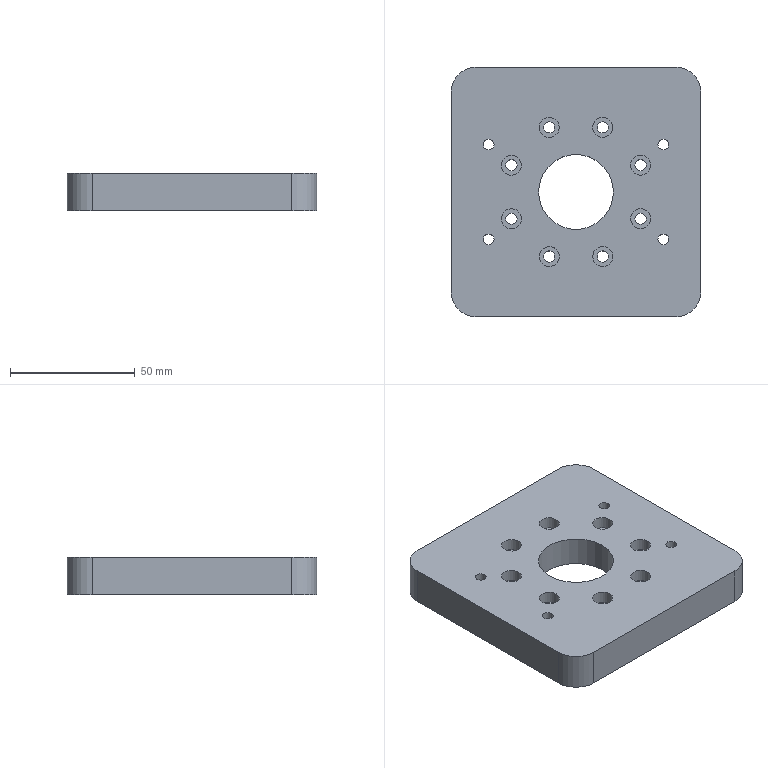Part | NX | 1 solid | 41 faces | box 100 x 100 x 15 mm | volume 127371 mm3 | cylinder 26 | plane 15 | commonest cylinder face diameters 4.5 x8 8 x8 4.3 x4 20 x4 30 x1 62.1 x1
STEP:
#1=CARTESIAN_POINT('',(-23.619,-10.715,-12.));
#2=VERTEX_POINT('',#1);
#3=CARTESIAN_POINT('',(-25.869,-10.715,-12.));
#4=DIRECTION('',(0.,0.,1.));
#5=DIRECTION('',(1.,0.,0.));
#6=AXIS2_PLACEMENT_3D('',#3,#4,#5);
#7=CIRCLE('',#6,2.25);
#8=EDGE_CURVE('',#2,#2,#7,.F.);
#9=ORIENTED_EDGE('',*,*,#8,.T.);
#10=EDGE_LOOP('',(#9));
#11=FACE_BOUND('',#10,.T.);
#12=CARTESIAN_POINT('',(-23.619,-10.715,-5.));
#13=VERTEX_POINT('',#12);
#14=CARTESIAN_POINT('',(-25.869,-10.715,-5.));
#15=DIRECTION('',(0.,0.,1.));
#16=DIRECTION('',(1.,0.,0.));
#17=AXIS2_PLACEMENT_3D('',#14,#15,#16);
#18=CIRCLE('',#17,2.25);
#19=EDGE_CURVE('',#13,#13,#18,.F.);
#20=ORIENTED_EDGE('',*,*,#19,.F.);
#21=EDGE_LOOP('',(#20));
#22=FACE_BOUND('',#21,.T.);
#23=CARTESIAN_POINT('',(-25.869,-10.715,-15.));
#24=DIRECTION('',(0.,0.,1.));
#25=DIRECTION('',(1.,0.,0.));
#26=AXIS2_PLACEMENT_3D('',#23,#24,#25);
#27=CYLINDRICAL_SURFACE('',#26,2.25);
#28=ADVANCED_FACE('',(#11,#22),#27,.F.);
#29=CARTESIAN_POINT('',(-23.619,10.715,-12.));
#30=VERTEX_POINT('',#29);
#31=CARTESIAN_POINT('',(-25.869,10.715,-12.));
#32=DIRECTION('',(0.,0.,1.));
#33=DIRECTION('',(1.,0.,0.));
#34=AXIS2_PLACEMENT_3D('',#31,#32,#33);
#35=CIRCLE('',#34,2.25);
#36=EDGE_CURVE('',#30,#30,#35,.F.);
#37=ORIENTED_EDGE('',*,*,#36,.T.);
#38=EDGE_LOOP('',(#37));
#39=FACE_BOUND('',#38,.T.);
#40=CARTESIAN_POINT('',(-23.619,10.715,-5.));
#41=VERTEX_POINT('',#40);
#42=CARTESIAN_POINT('',(-25.869,10.715,-5.));
#43=DIRECTION('',(0.,0.,1.));
#44=DIRECTION('',(1.,0.,0.));
#45=AXIS2_PLACEMENT_3D('',#42,#43,#44);
#46=CIRCLE('',#45,2.25);
#47=EDGE_CURVE('',#41,#41,#46,.F.);
#48=ORIENTED_EDGE('',*,*,#47,.F.);
#49=EDGE_LOOP('',(#48));
#50=FACE_BOUND('',#49,.T.);
#51=CARTESIAN_POINT('',(-25.869,10.715,-15.));
#52=DIRECTION('',(0.,0.,1.));
#53=DIRECTION('',(1.,0.,0.));
#54=AXIS2_PLACEMENT_3D('',#51,#52,#53);
#55=CYLINDRICAL_SURFACE('',#54,2.25);
#56=ADVANCED_FACE('',(#39,#50),#55,.F.);
#57=CARTESIAN_POINT('',(-8.465,-25.869,-12.));
#58=VERTEX_POINT('',#57);
#59=CARTESIAN_POINT('',(-10.715,-25.869,-12.));
#60=DIRECTION('',(0.,0.,1.));
#61=DIRECTION('',(1.,0.,0.));
#62=AXIS2_PLACEMENT_3D('',#59,#60,#61);
#63=CIRCLE('',#62,2.25);
#64=EDGE_CURVE('',#58,#58,#63,.F.);
#65=ORIENTED_EDGE('',*,*,#64,.T.);
#66=EDGE_LOOP('',(#65));
#67=FACE_BOUND('',#66,.T.);
#68=CARTESIAN_POINT('',(-8.465,-25.869,-5.));
#69=VERTEX_POINT('',#68);
#70=CARTESIAN_POINT('',(-10.715,-25.869,-5.));
#71=DIRECTION('',(0.,0.,1.));
#72=DIRECTION('',(1.,0.,0.));
#73=AXIS2_PLACEMENT_3D('',#70,#71,#72);
#74=CIRCLE('',#73,2.25);
#75=EDGE_CURVE('',#69,#69,#74,.F.);
#76=ORIENTED_EDGE('',*,*,#75,.F.);
#77=EDGE_LOOP('',(#76));
#78=FACE_BOUND('',#77,.T.);
#79=CARTESIAN_POINT('',(-10.715,-25.869,-15.));
#80=DIRECTION('',(0.,0.,1.));
#81=DIRECTION('',(1.,0.,0.));
#82=AXIS2_PLACEMENT_3D('',#79,#80,#81);
#83=CYLINDRICAL_SURFACE('',#82,2.25);
#84=ADVANCED_FACE('',(#67,#78),#83,.F.);
#85=CARTESIAN_POINT('',(-8.465,25.869,-12.));
#86=VERTEX_POINT('',#85);
#87=CARTESIAN_POINT('',(-10.715,25.869,-12.));
#88=DIRECTION('',(0.,0.,1.));
#89=DIRECTION('',(1.,0.,0.));
#90=AXIS2_PLACEMENT_3D('',#87,#88,#89);
#91=CIRCLE('',#90,2.25);
#92=EDGE_CURVE('',#86,#86,#91,.F.);
#93=ORIENTED_EDGE('',*,*,#92,.T.);
#94=EDGE_LOOP('',(#93));
#95=FACE_BOUND('',#94,.T.);
#96=CARTESIAN_POINT('',(-8.465,25.869,-5.));
#97=VERTEX_POINT('',#96);
#98=CARTESIAN_POINT('',(-10.715,25.869,-5.));
#99=DIRECTION('',(0.,0.,1.));
#100=DIRECTION('',(1.,0.,0.));
#101=AXIS2_PLACEMENT_3D('',#98,#99,#100);
#102=CIRCLE('',#101,2.25);
#103=EDGE_CURVE('',#97,#97,#102,.F.);
#104=ORIENTED_EDGE('',*,*,#103,.F.);
#105=EDGE_LOOP('',(#104));
#106=FACE_BOUND('',#105,.T.);
#107=CARTESIAN_POINT('',(-10.715,25.869,-15.));
#108=DIRECTION('',(0.,0.,1.));
#109=DIRECTION('',(1.,0.,0.));
#110=AXIS2_PLACEMENT_3D('',#107,#108,#109);
#111=CYLINDRICAL_SURFACE('',#110,2.25);
#112=ADVANCED_FACE('',(#95,#106),#111,.F.);
#113=CARTESIAN_POINT('',(12.965,-25.869,-12.));
#114=VERTEX_POINT('',#113);
#115=CARTESIAN_POINT('',(10.715,-25.869,-12.));
#116=DIRECTION('',(0.,0.,1.));
#117=DIRECTION('',(1.,0.,0.));
#118=AXIS2_PLACEMENT_3D('',#115,#116,#117);
#119=CIRCLE('',#118,2.25);
#120=EDGE_CURVE('',#114,#114,#119,.F.);
#121=ORIENTED_EDGE('',*,*,#120,.T.);
#122=EDGE_LOOP('',(#121));
#123=FACE_BOUND('',#122,.T.);
#124=CARTESIAN_POINT('',(12.965,-25.869,-5.));
#125=VERTEX_POINT('',#124);
#126=CARTESIAN_POINT('',(10.715,-25.869,-5.));
#127=DIRECTION('',(0.,0.,1.));
#128=DIRECTION('',(1.,0.,0.));
#129=AXIS2_PLACEMENT_3D('',#126,#127,#128);
#130=CIRCLE('',#129,2.25);
#131=EDGE_CURVE('',#125,#125,#130,.F.);
#132=ORIENTED_EDGE('',*,*,#131,.F.);
#133=EDGE_LOOP('',(#132));
#134=FACE_BOUND('',#133,.T.);
#135=CARTESIAN_POINT('',(10.715,-25.869,-15.));
#136=DIRECTION('',(0.,0.,1.));
#137=DIRECTION('',(1.,0.,0.));
#138=AXIS2_PLACEMENT_3D('',#135,#136,#137);
#139=CYLINDRICAL_SURFACE('',#138,2.25);
#140=ADVANCED_FACE('',(#123,#134),#139,.F.);
#141=CARTESIAN_POINT('',(12.965,25.869,-12.));
#142=VERTEX_POINT('',#141);
#143=CARTESIAN_POINT('',(10.715,25.869,-12.));
#144=DIRECTION('',(0.,0.,1.));
#145=DIRECTION('',(1.,0.,0.));
#146=AXIS2_PLACEMENT_3D('',#143,#144,#145);
#147=CIRCLE('',#146,2.25);
#148=EDGE_CURVE('',#142,#142,#147,.F.);
#149=ORIENTED_EDGE('',*,*,#148,.T.);
#150=EDGE_LOOP('',(#149));
#151=FACE_BOUND('',#150,.T.);
#152=CARTESIAN_POINT('',(12.965,25.869,-5.));
#153=VERTEX_POINT('',#152);
#154=CARTESIAN_POINT('',(10.715,25.869,-5.));
#155=DIRECTION('',(0.,0.,1.));
#156=DIRECTION('',(1.,0.,0.));
#157=AXIS2_PLACEMENT_3D('',#154,#155,#156);
#158=CIRCLE('',#157,2.25);
#159=EDGE_CURVE('',#153,#153,#158,.F.);
#160=ORIENTED_EDGE('',*,*,#159,.F.);
#161=EDGE_LOOP('',(#160));
#162=FACE_BOUND('',#161,.T.);
#163=CARTESIAN_POINT('',(10.715,25.869,-15.));
#164=DIRECTION('',(0.,0.,1.));
#165=DIRECTION('',(1.,0.,0.));
#166=AXIS2_PLACEMENT_3D('',#163,#164,#165);
#167=CYLINDRICAL_SURFACE('',#166,2.25);
#168=ADVANCED_FACE('',(#151,#162),#167,.F.);
#169=CARTESIAN_POINT('',(28.119,-10.715,-12.));
#170=VERTEX_POINT('',#169);
#171=CARTESIAN_POINT('',(25.869,-10.715,-12.));
#172=DIRECTION('',(0.,0.,1.));
#173=DIRECTION('',(1.,0.,0.));
#174=AXIS2_PLACEMENT_3D('',#171,#172,#173);
#175=CIRCLE('',#174,2.25);
#176=EDGE_CURVE('',#170,#170,#175,.F.);
#177=ORIENTED_EDGE('',*,*,#176,.T.);
#178=EDGE_LOOP('',(#177));
#179=FACE_BOUND('',#178,.T.);
#180=CARTESIAN_POINT('',(28.119,-10.715,-5.));
#181=VERTEX_POINT('',#180);
#182=CARTESIAN_POINT('',(25.869,-10.715,-5.));
#183=DIRECTION('',(0.,0.,1.));
#184=DIRECTION('',(1.,0.,0.));
#185=AXIS2_PLACEMENT_3D('',#182,#183,#184);
#186=CIRCLE('',#185,2.25);
#187=EDGE_CURVE('',#181,#181,#186,.F.);
#188=ORIENTED_EDGE('',*,*,#187,.F.);
#189=EDGE_LOOP('',(#188));
#190=FACE_BOUND('',#189,.T.);
#191=CARTESIAN_POINT('',(25.869,-10.715,-15.));
#192=DIRECTION('',(0.,0.,1.));
#193=DIRECTION('',(1.,0.,0.));
#194=AXIS2_PLACEMENT_3D('',#191,#192,#193);
#195=CYLINDRICAL_SURFACE('',#194,2.25);
#196=ADVANCED_FACE('',(#179,#190),#195,.F.);
#197=CARTESIAN_POINT('',(28.119,10.715,-12.));
#198=VERTEX_POINT('',#197);
#199=CARTESIAN_POINT('',(25.869,10.715,-12.));
#200=DIRECTION('',(0.,0.,1.));
#201=DIRECTION('',(1.,0.,0.));
#202=AXIS2_PLACEMENT_3D('',#199,#200,#201);
#203=CIRCLE('',#202,2.25);
#204=EDGE_CURVE('',#198,#198,#203,.F.);
#205=ORIENTED_EDGE('',*,*,#204,.T.);
#206=EDGE_LOOP('',(#205));
#207=FACE_BOUND('',#206,.T.);
#208=CARTESIAN_POINT('',(28.119,10.715,-5.));
#209=VERTEX_POINT('',#208);
#210=CARTESIAN_POINT('',(25.869,10.715,-5.));
#211=DIRECTION('',(0.,0.,1.));
#212=DIRECTION('',(1.,0.,0.));
#213=AXIS2_PLACEMENT_3D('',#210,#211,#212);
#214=CIRCLE('',#213,2.25);
#215=EDGE_CURVE('',#209,#209,#214,.F.);
#216=ORIENTED_EDGE('',*,*,#215,.F.);
#217=EDGE_LOOP('',(#216));
#218=FACE_BOUND('',#217,.T.);
#219=CARTESIAN_POINT('',(25.869,10.715,-15.));
#220=DIRECTION('',(0.,0.,1.));
#221=DIRECTION('',(1.,0.,0.));
#222=AXIS2_PLACEMENT_3D('',#219,#220,#221);
#223=CYLINDRICAL_SURFACE('',#222,2.25);
#224=ADVANCED_FACE('',(#207,#218),#223,.F.);
#225=CARTESIAN_POINT('',(-50.,-40.,0.));
#226=VERTEX_POINT('',#225);
#227=CARTESIAN_POINT('',(-50.,40.,0.));
#228=VERTEX_POINT('',#227);
#229=CARTESIAN_POINT('',(-50.,-50.,0.));
#230=DIRECTION('',(0.,1.,0.));
#231=VECTOR('',#230,1000.);
#232=LINE('',#229,#231);
#233=EDGE_CURVE('',#226,#228,#232,.T.);
#234=ORIENTED_EDGE('',*,*,#233,.T.);
#235=CARTESIAN_POINT('',(-50.,40.,-15.));
#236=VERTEX_POINT('',#235);
#237=CARTESIAN_POINT('',(-50.,40.,-15.));
#238=DIRECTION('',(0.,0.,1.));
#239=VECTOR('',#238,1000.);
#240=LINE('',#237,#239);
#241=EDGE_CURVE('',#228,#236,#240,.F.);
#242=ORIENTED_EDGE('',*,*,#241,.T.);
#243=CARTESIAN_POINT('',(-50.,-40.,-15.));
#244=VERTEX_POINT('',#243);
#245=CARTESIAN_POINT('',(-50.,-50.,-15.));
#246=DIRECTION('',(0.,1.,0.));
#247=VECTOR('',#246,1000.);
#248=LINE('',#245,#247);
#249=EDGE_CURVE('',#244,#236,#248,.T.);
#250=ORIENTED_EDGE('',*,*,#249,.F.);
#251=CARTESIAN_POINT('',(-50.,-40.,-15.));
#252=DIRECTION('',(0.,0.,1.));
#253=VECTOR('',#252,1000.);
#254=LINE('',#251,#253);
#255=EDGE_CURVE('',#244,#226,#254,.T.);
#256=ORIENTED_EDGE('',*,*,#255,.T.);
#257=EDGE_LOOP('',(#234,#242,#250,#256));
#258=FACE_BOUND('',#257,.T.);
#259=CARTESIAN_POINT('',(-50.,-50.,-15.));
#260=DIRECTION('',(1.,0.,0.));
#261=DIRECTION('',(0.,0.,-1.));
#262=AXIS2_PLACEMENT_3D('',#259,#260,#261);
#263=PLANE('',#262);
#264=ADVANCED_FACE('',(#258),#263,.F.);
#265=CARTESIAN_POINT('',(-40.,50.,-15.));
#266=VERTEX_POINT('',#265);
#267=CARTESIAN_POINT('',(40.,50.,-15.));
#268=VERTEX_POINT('',#267);
#269=CARTESIAN_POINT('',(-50.,50.,-15.));
#270=DIRECTION('',(1.,0.,0.));
#271=VECTOR('',#270,1000.);
#272=LINE('',#269,#271);
#273=EDGE_CURVE('',#266,#268,#272,.T.);
#274=ORIENTED_EDGE('',*,*,#273,.F.);
#275=CARTESIAN_POINT('',(-40.,50.,0.));
#276=VERTEX_POINT('',#275);
#277=CARTESIAN_POINT('',(-40.,50.,-15.));
#278=DIRECTION('',(0.,0.,1.));
#279=VECTOR('',#278,1000.);
#280=LINE('',#277,#279);
#281=EDGE_CURVE('',#266,#276,#280,.T.);
#282=ORIENTED_EDGE('',*,*,#281,.T.);
#283=CARTESIAN_POINT('',(40.,50.,0.));
#284=VERTEX_POINT('',#283);
#285=CARTESIAN_POINT('',(-50.,50.,0.));
#286=DIRECTION('',(1.,0.,0.));
#287=VECTOR('',#286,1000.);
#288=LINE('',#285,#287);
#289=EDGE_CURVE('',#276,#284,#288,.T.);
#290=ORIENTED_EDGE('',*,*,#289,.T.);
#291=CARTESIAN_POINT('',(40.,50.,-15.));
#292=DIRECTION('',(0.,0.,1.));
#293=VECTOR('',#292,1000.);
#294=LINE('',#291,#293);
#295=EDGE_CURVE('',#284,#268,#294,.F.);
#296=ORIENTED_EDGE('',*,*,#295,.T.);
#297=EDGE_LOOP('',(#274,#282,#290,#296));
#298=FACE_BOUND('',#297,.T.);
#299=CARTESIAN_POINT('',(-50.,50.,-15.));
#300=DIRECTION('',(0.,-1.,0.));
#301=DIRECTION('',(1.,0.,0.));
#302=AXIS2_PLACEMENT_3D('',#299,#300,#301);
#303=PLANE('',#302);
#304=ADVANCED_FACE('',(#298),#303,.F.);
#305=CARTESIAN_POINT('',(50.,40.,-15.));
#306=VERTEX_POINT('',#305);
#307=CARTESIAN_POINT('',(50.,-40.,-15.));
#308=VERTEX_POINT('',#307);
#309=CARTESIAN_POINT('',(50.,50.,-15.));
#310=DIRECTION('',(0.,-1.,0.));
#311=VECTOR('',#310,1000.);
#312=LINE('',#309,#311);
#313=EDGE_CURVE('',#306,#308,#312,.T.);
#314=ORIENTED_EDGE('',*,*,#313,.F.);
#315=CARTESIAN_POINT('',(50.,40.,0.));
#316=VERTEX_POINT('',#315);
#317=CARTESIAN_POINT('',(50.,40.,-15.));
#318=DIRECTION('',(0.,0.,1.));
#319=VECTOR('',#318,1000.);
#320=LINE('',#317,#319);
#321=EDGE_CURVE('',#306,#316,#320,.T.);
#322=ORIENTED_EDGE('',*,*,#321,.T.);
#323=CARTESIAN_POINT('',(50.,-40.,0.));
#324=VERTEX_POINT('',#323);
#325=CARTESIAN_POINT('',(50.,50.,0.));
#326=DIRECTION('',(0.,-1.,0.));
#327=VECTOR('',#326,1000.);
#328=LINE('',#325,#327);
#329=EDGE_CURVE('',#316,#324,#328,.T.);
#330=ORIENTED_EDGE('',*,*,#329,.T.);
#331=CARTESIAN_POINT('',(50.,-40.,-15.));
#332=DIRECTION('',(0.,0.,1.));
#333=VECTOR('',#332,1000.);
#334=LINE('',#331,#333);
#335=EDGE_CURVE('',#324,#308,#334,.F.);
#336=ORIENTED_EDGE('',*,*,#335,.T.);
#337=EDGE_LOOP('',(#314,#322,#330,#336));
#338=FACE_BOUND('',#337,.T.);
#339=CARTESIAN_POINT('',(50.,50.,-15.));
#340=DIRECTION('',(-1.,0.,0.));
#341=DIRECTION('',(0.,0.,1.));
#342=AXIS2_PLACEMENT_3D('',#339,#340,#341);
#343=PLANE('',#342);
#344=ADVANCED_FACE('',(#338),#343,.F.);
#345=CARTESIAN_POINT('',(-32.85,19.,-15.));
#346=VERTEX_POINT('',#345);
#347=CARTESIAN_POINT('',(-35.,19.,-15.));
#348=DIRECTION('',(0.,0.,1.));
#349=DIRECTION('',(1.,0.,0.));
#350=AXIS2_PLACEMENT_3D('',#347,#348,#349);
#351=CIRCLE('',#350,2.15);
#352=EDGE_CURVE('',#346,#346,#351,.T.);
#353=ORIENTED_EDGE('',*,*,#352,.F.);
#354=EDGE_LOOP('',(#353));
#355=FACE_BOUND('',#354,.T.);
#356=CARTESIAN_POINT('',(-32.85,19.,0.));
#357=VERTEX_POINT('',#356);
#358=CARTESIAN_POINT('',(-35.,19.,0.));
#359=DIRECTION('',(0.,0.,1.));
#360=DIRECTION('',(1.,0.,0.));
#361=AXIS2_PLACEMENT_3D('',#358,#359,#360);
#362=CIRCLE('',#361,2.15);
#363=EDGE_CURVE('',#357,#357,#362,.T.);
#364=ORIENTED_EDGE('',*,*,#363,.T.);
#365=EDGE_LOOP('',(#364));
#366=FACE_BOUND('',#365,.T.);
#367=CARTESIAN_POINT('',(-35.,19.,-15.));
#368=DIRECTION('',(0.,0.,1.));
#369=DIRECTION('',(1.,0.,0.));
#370=AXIS2_PLACEMENT_3D('',#367,#368,#369);
#371=CYLINDRICAL_SURFACE('',#370,2.15);
#372=ADVANCED_FACE('',(#355,#366),#371,.F.);
#373=CARTESIAN_POINT('',(15.,0.,-12.));
#374=VERTEX_POINT('',#373);
#375=CARTESIAN_POINT('',(0.,0.,-12.));
#376=DIRECTION('',(0.,0.,1.));
#377=DIRECTION('',(1.,0.,0.));
#378=AXIS2_PLACEMENT_3D('',#375,#376,#377);
#379=CIRCLE('',#378,15.);
#380=EDGE_CURVE('',#374,#374,#379,.F.);
#381=ORIENTED_EDGE('',*,*,#380,.T.);
#382=EDGE_LOOP('',(#381));
#383=FACE_BOUND('',#382,.T.);
#384=CARTESIAN_POINT('',(15.,0.,0.));
#385=VERTEX_POINT('',#384);
#386=CARTESIAN_POINT('',(0.,0.,0.));
#387=DIRECTION('',(0.,0.,1.));
#388=DIRECTION('',(1.,0.,0.));
#389=AXIS2_PLACEMENT_3D('',#386,#387,#388);
#390=CIRCLE('',#389,15.);
#391=EDGE_CURVE('',#385,#385,#390,.T.);
#392=ORIENTED_EDGE('',*,*,#391,.T.);
#393=EDGE_LOOP('',(#392));
#394=FACE_BOUND('',#393,.T.);
#395=CARTESIAN_POINT('',(0.,0.,-15.));
#396=DIRECTION('',(0.,0.,1.));
#397=DIRECTION('',(1.,0.,0.));
#398=AXIS2_PLACEMENT_3D('',#395,#396,#397);
#399=CYLINDRICAL_SURFACE('',#398,15.);
#400=ADVANCED_FACE('',(#383,#394),#399,.F.);
#401=CARTESIAN_POINT('',(37.15,-19.,-15.));
#402=VERTEX_POINT('',#401);
#403=CARTESIAN_POINT('',(35.,-19.,-15.));
#404=DIRECTION('',(0.,0.,1.));
#405=DIRECTION('',(1.,0.,0.));
#406=AXIS2_PLACEMENT_3D('',#403,#404,#405);
#407=CIRCLE('',#406,2.15);
#408=EDGE_CURVE('',#402,#402,#407,.T.);
#409=ORIENTED_EDGE('',*,*,#408,.F.);
#410=EDGE_LOOP('',(#409));
#411=FACE_BOUND('',#410,.T.);
#412=CARTESIAN_POINT('',(37.15,-19.,0.));
#413=VERTEX_POINT('',#412);
#414=CARTESIAN_POINT('',(35.,-19.,0.));
#415=DIRECTION('',(0.,0.,1.));
#416=DIRECTION('',(1.,0.,0.));
#417=AXIS2_PLACEMENT_3D('',#414,#415,#416);
#418=CIRCLE('',#417,2.15);
#419=EDGE_CURVE('',#413,#413,#418,.T.);
#420=ORIENTED_EDGE('',*,*,#419,.T.);
#421=EDGE_LOOP('',(#420));
#422=FACE_BOUND('',#421,.T.);
#423=CARTESIAN_POINT('',(35.,-19.,-15.));
#424=DIRECTION('',(0.,0.,1.));
#425=DIRECTION('',(1.,0.,0.));
#426=AXIS2_PLACEMENT_3D('',#423,#424,#425);
#427=CYLINDRICAL_SURFACE('',#426,2.15);
#428=ADVANCED_FACE('',(#411,#422),#427,.F.);
#429=CARTESIAN_POINT('',(37.15,19.,-15.));
#430=VERTEX_POINT('',#429);
#431=CARTESIAN_POINT('',(35.,19.,-15.));
#432=DIRECTION('',(0.,0.,1.));
#433=DIRECTION('',(1.,0.,0.));
#434=AXIS2_PLACEMENT_3D('',#431,#432,#433);
#435=CIRCLE('',#434,2.15);
#436=EDGE_CURVE('',#430,#430,#435,.T.);
#437=ORIENTED_EDGE('',*,*,#436,.F.);
#438=EDGE_LOOP('',(#437));
#439=FACE_BOUND('',#438,.T.);
#440=CARTESIAN_POINT('',(37.15,19.,0.));
#441=VERTEX_POINT('',#440);
#442=CARTESIAN_POINT('',(35.,19.,0.));
#443=DIRECTION('',(0.,0.,1.));
#444=DIRECTION('',(1.,0.,0.));
#445=AXIS2_PLACEMENT_3D('',#442,#443,#444);
#446=CIRCLE('',#445,2.15);
#447=EDGE_CURVE('',#441,#441,#446,.T.);
#448=ORIENTED_EDGE('',*,*,#447,.T.);
#449=EDGE_LOOP('',(#448));
#450=FACE_BOUND('',#449,.T.);
#451=CARTESIAN_POINT('',(35.,19.,-15.));
#452=DIRECTION('',(0.,0.,1.));
#453=DIRECTION('',(1.,0.,0.));
#454=AXIS2_PLACEMENT_3D('',#451,#452,#453);
#455=CYLINDRICAL_SURFACE('',#454,2.15);
#456=ADVANCED_FACE('',(#439,#450),#455,.F.);
#457=CARTESIAN_POINT('',(40.,-50.,0.));
#458=VERTEX_POINT('',#457);
#459=CARTESIAN_POINT('',(-40.,-50.,0.));
#460=VERTEX_POINT('',#459);
#461=CARTESIAN_POINT('',(50.,-50.,0.));
#462=DIRECTION('',(-1.,0.,0.));
#463=VECTOR('',#462,1000.);
#464=LINE('',#461,#463);
#465=EDGE_CURVE('',#458,#460,#464,.T.);
#466=ORIENTED_EDGE('',*,*,#465,.T.);
#467=CARTESIAN_POINT('',(-40.,-50.,-15.));
#468=VERTEX_POINT('',#467);
#469=CARTESIAN_POINT('',(-40.,-50.,-15.));
#470=DIRECTION('',(0.,0.,1.));
#471=VECTOR('',#470,1000.);
#472=LINE('',#469,#471);
#473=EDGE_CURVE('',#460,#468,#472,.F.);
#474=ORIENTED_EDGE('',*,*,#473,.T.);
#475=CARTESIAN_POINT('',(40.,-50.,-15.));
#476=VERTEX_POINT('',#475);
#477=CARTESIAN_POINT('',(50.,-50.,-15.));
#478=DIRECTION('',(-1.,0.,0.));
#479=VECTOR('',#478,1000.);
#480=LINE('',#477,#479);
#481=EDGE_CURVE('',#476,#468,#480,.T.);
#482=ORIENTED_EDGE('',*,*,#481,.F.);
#483=CARTESIAN_POINT('',(40.,-50.,-15.));
#484=DIRECTION('',(0.,0.,1.));
#485=VECTOR('',#484,1000.);
#486=LINE('',#483,#485);
#487=EDGE_CURVE('',#476,#458,#486,.T.);
#488=ORIENTED_EDGE('',*,*,#487,.T.);
#489=EDGE_LOOP('',(#466,#474,#482,#488));
#490=FACE_BOUND('',#489,.T.);
#491=CARTESIAN_POINT('',(50.,-50.,-15.));
#492=DIRECTION('',(0.,1.,0.));
#493=DIRECTION('',(-1.,0.,0.));
#494=AXIS2_PLACEMENT_3D('',#491,#492,#493);
#495=PLANE('',#494);
#496=ADVANCED_FACE('',(#490),#495,.F.);
#497=CARTESIAN_POINT('',(-32.85,-19.,-15.));
#498=VERTEX_POINT('',#497);
#499=CARTESIAN_POINT('',(-35.,-19.,-15.));
#500=DIRECTION('',(0.,0.,1.));
#501=DIRECTION('',(1.,0.,0.));
#502=AXIS2_PLACEMENT_3D('',#499,#500,#501);
#503=CIRCLE('',#502,2.15);
#504=EDGE_CURVE('',#498,#498,#503,.T.);
#505=ORIENTED_EDGE('',*,*,#504,.F.);
#506=EDGE_LOOP('',(#505));
#507=FACE_BOUND('',#506,.T.);
#508=CARTESIAN_POINT('',(-32.85,-19.,0.));
#509=VERTEX_POINT('',#508);
#510=CARTESIAN_POINT('',(-35.,-19.,0.));
#511=DIRECTION('',(0.,0.,1.));
#512=DIRECTION('',(1.,0.,0.));
#513=AXIS2_PLACEMENT_3D('',#510,#511,#512);
#514=CIRCLE('',#513,2.15);
#515=EDGE_CURVE('',#509,#509,#514,.T.);
#516=ORIENTED_EDGE('',*,*,#515,.T.);
#517=EDGE_LOOP('',(#516));
#518=FACE_BOUND('',#517,.T.);
#519=CARTESIAN_POINT('',(-35.,-19.,-15.));
#520=DIRECTION('',(0.,0.,1.));
#521=DIRECTION('',(1.,0.,0.));
#522=AXIS2_PLACEMENT_3D('',#519,#520,#521);
#523=CYLINDRICAL_SURFACE('',#522,2.15);
#524=ADVANCED_FACE('',(#507,#518),#523,.F.);
#525=CARTESIAN_POINT('',(31.05,0.,-15.));
#526=VERTEX_POINT('',#525);
#527=CARTESIAN_POINT('',(0.,0.,-15.));
#528=DIRECTION('',(0.,0.,1.));
#529=DIRECTION('',(1.,0.,0.));
#530=AXIS2_PLACEMENT_3D('',#527,#528,#529);
#531=CIRCLE('',#530,31.05);
#532=EDGE_CURVE('',#526,#526,#531,.T.);
#533=ORIENTED_EDGE('',*,*,#532,.T.);
#534=EDGE_LOOP('',(#533));
#535=FACE_BOUND('',#534,.T.);
#536=ORIENTED_EDGE('',*,*,#249,.T.);
#537=CARTESIAN_POINT('',(-40.,40.,-15.));
#538=DIRECTION('',(0.,0.,1.));
#539=DIRECTION('',(1.,0.,0.));
#540=AXIS2_PLACEMENT_3D('',#537,#538,#539);
#541=CIRCLE('',#540,10.);
#542=EDGE_CURVE('',#236,#266,#541,.F.);
#543=ORIENTED_EDGE('',*,*,#542,.T.);
#544=ORIENTED_EDGE('',*,*,#273,.T.);
#545=CARTESIAN_POINT('',(40.,40.,-15.));
#546=DIRECTION('',(0.,0.,1.));
#547=DIRECTION('',(1.,0.,0.));
#548=AXIS2_PLACEMENT_3D('',#545,#546,#547);
#549=CIRCLE('',#548,10.);
#550=EDGE_CURVE('',#268,#306,#549,.F.);
#551=ORIENTED_EDGE('',*,*,#550,.T.);
#552=ORIENTED_EDGE('',*,*,#313,.T.);
#553=CARTESIAN_POINT('',(40.,-40.,-15.));
#554=DIRECTION('',(0.,0.,1.));
#555=DIRECTION('',(1.,0.,0.));
#556=AXIS2_PLACEMENT_3D('',#553,#554,#555);
#557=CIRCLE('',#556,10.);
#558=EDGE_CURVE('',#308,#476,#557,.F.);
#559=ORIENTED_EDGE('',*,*,#558,.T.);
#560=ORIENTED_EDGE('',*,*,#481,.T.);
#561=CARTESIAN_POINT('',(-40.,-40.,-15.));
#562=DIRECTION('',(0.,0.,1.));
#563=DIRECTION('',(1.,0.,0.));
#564=AXIS2_PLACEMENT_3D('',#561,#562,#563);
#565=CIRCLE('',#564,10.);
#566=EDGE_CURVE('',#468,#244,#565,.F.);
#567=ORIENTED_EDGE('',*,*,#566,.T.);
#568=EDGE_LOOP('',(#536,#543,#544,#551,#552,#559,#560,#567));
#569=FACE_BOUND('',#568,.T.);
#570=ORIENTED_EDGE('',*,*,#436,.T.);
#571=EDGE_LOOP('',(#570));
#572=FACE_BOUND('',#571,.T.);
#573=ORIENTED_EDGE('',*,*,#408,.T.);
#574=EDGE_LOOP('',(#573));
#575=FACE_BOUND('',#574,.T.);
#576=ORIENTED_EDGE('',*,*,#352,.T.);
#577=EDGE_LOOP('',(#576));
#578=FACE_BOUND('',#577,.T.);
#579=ORIENTED_EDGE('',*,*,#504,.T.);
#580=EDGE_LOOP('',(#579));
#581=FACE_BOUND('',#580,.T.);
#582=CARTESIAN_POINT('',(35.,19.,-15.));
#583=DIRECTION('',(0.,0.,1.));
#584=DIRECTION('',(1.,0.,0.));
#585=AXIS2_PLACEMENT_3D('',#582,#583,#584);
#586=PLANE('',#585);
#587=ADVANCED_FACE('',(#535,#569,#572,#575,#578,#581),#586,.F.);
#588=CARTESIAN_POINT('',(-10.715,21.869,0.));
#589=VERTEX_POINT('',#588);
#590=CARTESIAN_POINT('',(-10.715,25.869,0.));
#591=DIRECTION('',(0.,0.,1.));
#592=DIRECTION('',(0.,-1.,0.));
#593=AXIS2_PLACEMENT_3D('',#590,#591,#592);
#594=CIRCLE('',#593,4.);
#595=EDGE_CURVE('',#589,#589,#594,.T.);
#596=ORIENTED_EDGE('',*,*,#595,.F.);
#597=EDGE_LOOP('',(#596));
#598=FACE_BOUND('',#597,.T.);
#599=CARTESIAN_POINT('',(10.715,-21.869,0.));
#600=VERTEX_POINT('',#599);
#601=CARTESIAN_POINT('',(10.715,-25.869,0.));
#602=DIRECTION('',(0.,0.,1.));
#603=DIRECTION('',(0.,1.,0.));
#604=AXIS2_PLACEMENT_3D('',#601,#602,#603);
#605=CIRCLE('',#604,4.);
#606=EDGE_CURVE('',#600,#600,#605,.T.);
#607=ORIENTED_EDGE('',*,*,#606,.F.);
#608=EDGE_LOOP('',(#607));
#609=FACE_BOUND('',#608,.T.);
#610=CARTESIAN_POINT('',(7.887,23.04,0.));
#611=VERTEX_POINT('',#610);
#612=CARTESIAN_POINT('',(10.715,25.869,0.));
#613=DIRECTION('',(0.,0.,1.));
#614=DIRECTION('',(-0.7071,-0.7071,0.));
#615=AXIS2_PLACEMENT_3D('',#612,#613,#614);
#616=CIRCLE('',#615,4.);
#617=EDGE_CURVE('',#611,#611,#616,.T.);
#618=ORIENTED_EDGE('',*,*,#617,.F.);
#619=EDGE_LOOP('',(#618));
#620=FACE_BOUND('',#619,.T.);
#621=CARTESIAN_POINT('',(23.04,-7.887,0.));
#622=VERTEX_POINT('',#621);
#623=CARTESIAN_POINT('',(25.869,-10.715,0.));
#624=DIRECTION('',(0.,0.,1.));
#625=DIRECTION('',(-0.7071,0.7071,0.));
#626=AXIS2_PLACEMENT_3D('',#623,#624,#625);
#627=CIRCLE('',#626,4.);
#628=EDGE_CURVE('',#622,#622,#627,.T.);
#629=ORIENTED_EDGE('',*,*,#628,.F.);
#630=EDGE_LOOP('',(#629));
#631=FACE_BOUND('',#630,.T.);
#632=CARTESIAN_POINT('',(-21.869,-10.715,0.));
#633=VERTEX_POINT('',#632);
#634=CARTESIAN_POINT('',(-25.869,-10.715,0.));
#635=DIRECTION('',(0.,0.,1.));
#636=DIRECTION('',(1.,0.,0.));
#637=AXIS2_PLACEMENT_3D('',#634,#635,#636);
#638=CIRCLE('',#637,4.);
#639=EDGE_CURVE('',#633,#633,#638,.T.);
#640=ORIENTED_EDGE('',*,*,#639,.F.);
#641=EDGE_LOOP('',(#640));
#642=FACE_BOUND('',#641,.T.);
#643=CARTESIAN_POINT('',(-23.04,7.887,0.));
#644=VERTEX_POINT('',#643);
#645=CARTESIAN_POINT('',(-25.869,10.715,0.));
#646=DIRECTION('',(0.,0.,1.));
#647=DIRECTION('',(0.7071,-0.7071,0.));
#648=AXIS2_PLACEMENT_3D('',#645,#646,#647);
#649=CIRCLE('',#648,4.);
#650=EDGE_CURVE('',#644,#644,#649,.T.);
#651=ORIENTED_EDGE('',*,*,#650,.F.);
#652=EDGE_LOOP('',(#651));
#653=FACE_BOUND('',#652,.T.);
#654=CARTESIAN_POINT('',(-7.887,-23.04,0.));
#655=VERTEX_POINT('',#654);
#656=CARTESIAN_POINT('',(-10.715,-25.869,0.));
#657=DIRECTION('',(0.,0.,1.));
#658=DIRECTION('',(0.7071,0.7071,0.));
#659=AXIS2_PLACEMENT_3D('',#656,#657,#658);
#660=CIRCLE('',#659,4.);
#661=EDGE_CURVE('',#655,#655,#660,.T.);
#662=ORIENTED_EDGE('',*,*,#661,.F.);
#663=EDGE_LOOP('',(#662));
#664=FACE_BOUND('',#663,.T.);
#665=CARTESIAN_POINT('',(21.869,10.715,0.));
#666=VERTEX_POINT('',#665);
#667=CARTESIAN_POINT('',(25.869,10.715,0.));
#668=DIRECTION('',(0.,0.,1.));
#669=DIRECTION('',(-1.,0.,0.));
#670=AXIS2_PLACEMENT_3D('',#667,#668,#669);
#671=CIRCLE('',#670,4.);
#672=EDGE_CURVE('',#666,#666,#671,.T.);
#673=ORIENTED_EDGE('',*,*,#672,.F.);
#674=EDGE_LOOP('',(#673));
#675=FACE_BOUND('',#674,.T.);
#676=ORIENTED_EDGE('',*,*,#289,.F.);
#677=CARTESIAN_POINT('',(-40.,40.,0.));
#678=DIRECTION('',(0.,0.,1.));
#679=DIRECTION('',(1.,0.,0.));
#680=AXIS2_PLACEMENT_3D('',#677,#678,#679);
#681=CIRCLE('',#680,10.);
#682=EDGE_CURVE('',#276,#228,#681,.T.);
#683=ORIENTED_EDGE('',*,*,#682,.T.);
#684=ORIENTED_EDGE('',*,*,#233,.F.);
#685=CARTESIAN_POINT('',(-40.,-40.,0.));
#686=DIRECTION('',(0.,0.,1.));
#687=DIRECTION('',(1.,0.,0.));
#688=AXIS2_PLACEMENT_3D('',#685,#686,#687);
#689=CIRCLE('',#688,10.);
#690=EDGE_CURVE('',#226,#460,#689,.T.);
#691=ORIENTED_EDGE('',*,*,#690,.T.);
#692=ORIENTED_EDGE('',*,*,#465,.F.);
#693=CARTESIAN_POINT('',(40.,-40.,0.));
#694=DIRECTION('',(0.,0.,1.));
#695=DIRECTION('',(1.,0.,0.));
#696=AXIS2_PLACEMENT_3D('',#693,#694,#695);
#697=CIRCLE('',#696,10.);
#698=EDGE_CURVE('',#458,#324,#697,.T.);
#699=ORIENTED_EDGE('',*,*,#698,.T.);
#700=ORIENTED_EDGE('',*,*,#329,.F.);
#701=CARTESIAN_POINT('',(40.,40.,0.));
#702=DIRECTION('',(0.,0.,1.));
#703=DIRECTION('',(1.,0.,0.));
#704=AXIS2_PLACEMENT_3D('',#701,#702,#703);
#705=CIRCLE('',#704,10.);
#706=EDGE_CURVE('',#316,#284,#705,.T.);
#707=ORIENTED_EDGE('',*,*,#706,.T.);
#708=EDGE_LOOP('',(#676,#683,#684,#691,#692,#699,#700,#707));
#709=FACE_BOUND('',#708,.T.);
#710=ORIENTED_EDGE('',*,*,#447,.F.);
#711=EDGE_LOOP('',(#710));
#712=FACE_BOUND('',#711,.T.);
#713=ORIENTED_EDGE('',*,*,#419,.F.);
#714=EDGE_LOOP('',(#713));
#715=FACE_BOUND('',#714,.T.);
#716=ORIENTED_EDGE('',*,*,#391,.F.);
#717=EDGE_LOOP('',(#716));
#718=FACE_BOUND('',#717,.T.);
#719=ORIENTED_EDGE('',*,*,#363,.F.);
#720=EDGE_LOOP('',(#719));
#721=FACE_BOUND('',#720,.T.);
#722=ORIENTED_EDGE('',*,*,#515,.F.);
#723=EDGE_LOOP('',(#722));
#724=FACE_BOUND('',#723,.T.);
#725=CARTESIAN_POINT('',(35.,19.,0.));
#726=DIRECTION('',(0.,0.,1.));
#727=DIRECTION('',(1.,0.,0.));
#728=AXIS2_PLACEMENT_3D('',#725,#726,#727);
#729=PLANE('',#728);
#730=ADVANCED_FACE('',(#598,#609,#620,#631,#642,#653,#664,#675,#709,#712,#715,#718,#721,#724),#729,.T.);
#731=CARTESIAN_POINT('',(21.869,10.715,-5.));
#732=VERTEX_POINT('',#731);
#733=CARTESIAN_POINT('',(25.869,10.715,-5.));
#734=DIRECTION('',(0.,0.,1.));
#735=DIRECTION('',(-1.,0.,0.));
#736=AXIS2_PLACEMENT_3D('',#733,#734,#735);
#737=CIRCLE('',#736,4.);
#738=EDGE_CURVE('',#732,#732,#737,.F.);
#739=ORIENTED_EDGE('',*,*,#738,.F.);
#740=EDGE_LOOP('',(#739));
#741=FACE_BOUND('',#740,.T.);
#742=ORIENTED_EDGE('',*,*,#215,.T.);
#743=EDGE_LOOP('',(#742));
#744=FACE_BOUND('',#743,.T.);
#745=CARTESIAN_POINT('',(25.869,10.715,-5.));
#746=DIRECTION('',(0.,0.,1.));
#747=DIRECTION('',(1.,0.,0.));
#748=AXIS2_PLACEMENT_3D('',#745,#746,#747);
#749=PLANE('',#748);
#750=ADVANCED_FACE('',(#741,#744),#749,.T.);
#751=ORIENTED_EDGE('',*,*,#738,.T.);
#752=EDGE_LOOP('',(#751));
#753=FACE_BOUND('',#752,.T.);
#754=ORIENTED_EDGE('',*,*,#672,.T.);
#755=EDGE_LOOP('',(#754));
#756=FACE_BOUND('',#755,.T.);
#757=CARTESIAN_POINT('',(25.869,10.715,-5.));
#758=DIRECTION('',(0.,0.,1.));
#759=DIRECTION('',(1.,0.,0.));
#760=AXIS2_PLACEMENT_3D('',#757,#758,#759);
#761=CYLINDRICAL_SURFACE('',#760,4.);
#762=ADVANCED_FACE('',(#753,#756),#761,.F.);
#763=CARTESIAN_POINT('',(-7.887,-23.04,-5.));
#764=VERTEX_POINT('',#763);
#765=CARTESIAN_POINT('',(-10.715,-25.869,-5.));
#766=DIRECTION('',(0.,0.,1.));
#767=DIRECTION('',(0.7071,0.7071,0.));
#768=AXIS2_PLACEMENT_3D('',#765,#766,#767);
#769=CIRCLE('',#768,4.);
#770=EDGE_CURVE('',#764,#764,#769,.F.);
#771=ORIENTED_EDGE('',*,*,#770,.F.);
#772=EDGE_LOOP('',(#771));
#773=FACE_BOUND('',#772,.T.);
#774=ORIENTED_EDGE('',*,*,#75,.T.);
#775=EDGE_LOOP('',(#774));
#776=FACE_BOUND('',#775,.T.);
#777=CARTESIAN_POINT('',(-10.715,-25.869,-5.));
#778=DIRECTION('',(0.,0.,1.));
#779=DIRECTION('',(1.,0.,0.));
#780=AXIS2_PLACEMENT_3D('',#777,#778,#779);
#781=PLANE('',#780);
#782=ADVANCED_FACE('',(#773,#776),#781,.T.);
#783=ORIENTED_EDGE('',*,*,#770,.T.);
#784=EDGE_LOOP('',(#783));
#785=FACE_BOUND('',#784,.T.);
#786=ORIENTED_EDGE('',*,*,#661,.T.);
#787=EDGE_LOOP('',(#786));
#788=FACE_BOUND('',#787,.T.);
#789=CARTESIAN_POINT('',(-10.715,-25.869,-5.));
#790=DIRECTION('',(0.,0.,1.));
#791=DIRECTION('',(1.,0.,0.));
#792=AXIS2_PLACEMENT_3D('',#789,#790,#791);
#793=CYLINDRICAL_SURFACE('',#792,4.);
#794=ADVANCED_FACE('',(#785,#788),#793,.F.);
#795=CARTESIAN_POINT('',(-23.04,7.887,-5.));
#796=VERTEX_POINT('',#795);
#797=CARTESIAN_POINT('',(-25.869,10.715,-5.));
#798=DIRECTION('',(0.,0.,1.));
#799=DIRECTION('',(0.7071,-0.7071,0.));
#800=AXIS2_PLACEMENT_3D('',#797,#798,#799);
#801=CIRCLE('',#800,4.);
#802=EDGE_CURVE('',#796,#796,#801,.F.);
#803=ORIENTED_EDGE('',*,*,#802,.F.);
#804=EDGE_LOOP('',(#803));
#805=FACE_BOUND('',#804,.T.);
#806=ORIENTED_EDGE('',*,*,#47,.T.);
#807=EDGE_LOOP('',(#806));
#808=FACE_BOUND('',#807,.T.);
#809=CARTESIAN_POINT('',(-25.869,10.715,-5.));
#810=DIRECTION('',(0.,0.,1.));
#811=DIRECTION('',(1.,0.,0.));
#812=AXIS2_PLACEMENT_3D('',#809,#810,#811);
#813=PLANE('',#812);
#814=ADVANCED_FACE('',(#805,#808),#813,.T.);
#815=ORIENTED_EDGE('',*,*,#802,.T.);
#816=EDGE_LOOP('',(#815));
#817=FACE_BOUND('',#816,.T.);
#818=ORIENTED_EDGE('',*,*,#650,.T.);
#819=EDGE_LOOP('',(#818));
#820=FACE_BOUND('',#819,.T.);
#821=CARTESIAN_POINT('',(-25.869,10.715,-5.));
#822=DIRECTION('',(0.,0.,1.));
#823=DIRECTION('',(1.,0.,0.));
#824=AXIS2_PLACEMENT_3D('',#821,#822,#823);
#825=CYLINDRICAL_SURFACE('',#824,4.);
#826=ADVANCED_FACE('',(#817,#820),#825,.F.);
#827=CARTESIAN_POINT('',(-21.869,-10.715,-5.));
#828=VERTEX_POINT('',#827);
#829=CARTESIAN_POINT('',(-25.869,-10.715,-5.));
#830=DIRECTION('',(0.,0.,1.));
#831=DIRECTION('',(1.,0.,0.));
#832=AXIS2_PLACEMENT_3D('',#829,#830,#831);
#833=CIRCLE('',#832,4.);
#834=EDGE_CURVE('',#828,#828,#833,.F.);
#835=ORIENTED_EDGE('',*,*,#834,.F.);
#836=EDGE_LOOP('',(#835));
#837=FACE_BOUND('',#836,.T.);
#838=ORIENTED_EDGE('',*,*,#19,.T.);
#839=EDGE_LOOP('',(#838));
#840=FACE_BOUND('',#839,.T.);
#841=CARTESIAN_POINT('',(-25.869,-10.715,-5.));
#842=DIRECTION('',(0.,0.,1.));
#843=DIRECTION('',(1.,0.,0.));
#844=AXIS2_PLACEMENT_3D('',#841,#842,#843);
#845=PLANE('',#844);
#846=ADVANCED_FACE('',(#837,#840),#845,.T.);
#847=ORIENTED_EDGE('',*,*,#834,.T.);
#848=EDGE_LOOP('',(#847));
#849=FACE_BOUND('',#848,.T.);
#850=ORIENTED_EDGE('',*,*,#639,.T.);
#851=EDGE_LOOP('',(#850));
#852=FACE_BOUND('',#851,.T.);
#853=CARTESIAN_POINT('',(-25.869,-10.715,-5.));
#854=DIRECTION('',(0.,0.,1.));
#855=DIRECTION('',(1.,0.,0.));
#856=AXIS2_PLACEMENT_3D('',#853,#854,#855);
#857=CYLINDRICAL_SURFACE('',#856,4.);
#858=ADVANCED_FACE('',(#849,#852),#857,.F.);
#859=CARTESIAN_POINT('',(23.04,-7.887,-5.));
#860=VERTEX_POINT('',#859);
#861=CARTESIAN_POINT('',(25.869,-10.715,-5.));
#862=DIRECTION('',(0.,0.,1.));
#863=DIRECTION('',(-0.7071,0.7071,0.));
#864=AXIS2_PLACEMENT_3D('',#861,#862,#863);
#865=CIRCLE('',#864,4.);
#866=EDGE_CURVE('',#860,#860,#865,.F.);
#867=ORIENTED_EDGE('',*,*,#866,.F.);
#868=EDGE_LOOP('',(#867));
#869=FACE_BOUND('',#868,.T.);
#870=ORIENTED_EDGE('',*,*,#187,.T.);
#871=EDGE_LOOP('',(#870));
#872=FACE_BOUND('',#871,.T.);
#873=CARTESIAN_POINT('',(25.869,-10.715,-5.));
#874=DIRECTION('',(0.,0.,1.));
#875=DIRECTION('',(1.,0.,0.));
#876=AXIS2_PLACEMENT_3D('',#873,#874,#875);
#877=PLANE('',#876);
#878=ADVANCED_FACE('',(#869,#872),#877,.T.);
#879=ORIENTED_EDGE('',*,*,#866,.T.);
#880=EDGE_LOOP('',(#879));
#881=FACE_BOUND('',#880,.T.);
#882=ORIENTED_EDGE('',*,*,#628,.T.);
#883=EDGE_LOOP('',(#882));
#884=FACE_BOUND('',#883,.T.);
#885=CARTESIAN_POINT('',(25.869,-10.715,-5.));
#886=DIRECTION('',(0.,0.,1.));
#887=DIRECTION('',(1.,0.,0.));
#888=AXIS2_PLACEMENT_3D('',#885,#886,#887);
#889=CYLINDRICAL_SURFACE('',#888,4.);
#890=ADVANCED_FACE('',(#881,#884),#889,.F.);
#891=CARTESIAN_POINT('',(7.887,23.04,-5.));
#892=VERTEX_POINT('',#891);
#893=CARTESIAN_POINT('',(10.715,25.869,-5.));
#894=DIRECTION('',(0.,0.,1.));
#895=DIRECTION('',(-0.7071,-0.7071,0.));
#896=AXIS2_PLACEMENT_3D('',#893,#894,#895);
#897=CIRCLE('',#896,4.);
#898=EDGE_CURVE('',#892,#892,#897,.F.);
#899=ORIENTED_EDGE('',*,*,#898,.F.);
#900=EDGE_LOOP('',(#899));
#901=FACE_BOUND('',#900,.T.);
#902=ORIENTED_EDGE('',*,*,#159,.T.);
#903=EDGE_LOOP('',(#902));
#904=FACE_BOUND('',#903,.T.);
#905=CARTESIAN_POINT('',(10.715,25.869,-5.));
#906=DIRECTION('',(0.,0.,1.));
#907=DIRECTION('',(1.,0.,0.));
#908=AXIS2_PLACEMENT_3D('',#905,#906,#907);
#909=PLANE('',#908);
#910=ADVANCED_FACE('',(#901,#904),#909,.T.);
#911=ORIENTED_EDGE('',*,*,#898,.T.);
#912=EDGE_LOOP('',(#911));
#913=FACE_BOUND('',#912,.T.);
#914=ORIENTED_EDGE('',*,*,#617,.T.);
#915=EDGE_LOOP('',(#914));
#916=FACE_BOUND('',#915,.T.);
#917=CARTESIAN_POINT('',(10.715,25.869,-5.));
#918=DIRECTION('',(0.,0.,1.));
#919=DIRECTION('',(1.,0.,0.));
#920=AXIS2_PLACEMENT_3D('',#917,#918,#919);
#921=CYLINDRICAL_SURFACE('',#920,4.);
#922=ADVANCED_FACE('',(#913,#916),#921,.F.);
#923=CARTESIAN_POINT('',(10.715,-21.869,-5.));
#924=VERTEX_POINT('',#923);
#925=CARTESIAN_POINT('',(10.715,-25.869,-5.));
#926=DIRECTION('',(0.,0.,1.));
#927=DIRECTION('',(0.,1.,0.));
#928=AXIS2_PLACEMENT_3D('',#925,#926,#927);
#929=CIRCLE('',#928,4.);
#930=EDGE_CURVE('',#924,#924,#929,.F.);
#931=ORIENTED_EDGE('',*,*,#930,.F.);
#932=EDGE_LOOP('',(#931));
#933=FACE_BOUND('',#932,.T.);
#934=ORIENTED_EDGE('',*,*,#131,.T.);
#935=EDGE_LOOP('',(#934));
#936=FACE_BOUND('',#935,.T.);
#937=CARTESIAN_POINT('',(10.715,-25.869,-5.));
#938=DIRECTION('',(0.,0.,1.));
#939=DIRECTION('',(1.,0.,0.));
#940=AXIS2_PLACEMENT_3D('',#937,#938,#939);
#941=PLANE('',#940);
#942=ADVANCED_FACE('',(#933,#936),#941,.T.);
#943=ORIENTED_EDGE('',*,*,#930,.T.);
#944=EDGE_LOOP('',(#943));
#945=FACE_BOUND('',#944,.T.);
#946=ORIENTED_EDGE('',*,*,#606,.T.);
#947=EDGE_LOOP('',(#946));
#948=FACE_BOUND('',#947,.T.);
#949=CARTESIAN_POINT('',(10.715,-25.869,-5.));
#950=DIRECTION('',(0.,0.,1.));
#951=DIRECTION('',(1.,0.,0.));
#952=AXIS2_PLACEMENT_3D('',#949,#950,#951);
#953=CYLINDRICAL_SURFACE('',#952,4.);
#954=ADVANCED_FACE('',(#945,#948),#953,.F.);
#955=CARTESIAN_POINT('',(-10.715,21.869,-5.));
#956=VERTEX_POINT('',#955);
#957=CARTESIAN_POINT('',(-10.715,25.869,-5.));
#958=DIRECTION('',(0.,0.,1.));
#959=DIRECTION('',(0.,-1.,0.));
#960=AXIS2_PLACEMENT_3D('',#957,#958,#959);
#961=CIRCLE('',#960,4.);
#962=EDGE_CURVE('',#956,#956,#961,.F.);
#963=ORIENTED_EDGE('',*,*,#962,.F.);
#964=EDGE_LOOP('',(#963));
#965=FACE_BOUND('',#964,.T.);
#966=ORIENTED_EDGE('',*,*,#103,.T.);
#967=EDGE_LOOP('',(#966));
#968=FACE_BOUND('',#967,.T.);
#969=CARTESIAN_POINT('',(-10.715,25.869,-5.));
#970=DIRECTION('',(0.,0.,1.));
#971=DIRECTION('',(1.,0.,0.));
#972=AXIS2_PLACEMENT_3D('',#969,#970,#971);
#973=PLANE('',#972);
#974=ADVANCED_FACE('',(#965,#968),#973,.T.);
#975=ORIENTED_EDGE('',*,*,#962,.T.);
#976=EDGE_LOOP('',(#975));
#977=FACE_BOUND('',#976,.T.);
#978=ORIENTED_EDGE('',*,*,#595,.T.);
#979=EDGE_LOOP('',(#978));
#980=FACE_BOUND('',#979,.T.);
#981=CARTESIAN_POINT('',(-10.715,25.869,-5.));
#982=DIRECTION('',(0.,0.,1.));
#983=DIRECTION('',(1.,0.,0.));
#984=AXIS2_PLACEMENT_3D('',#981,#982,#983);
#985=CYLINDRICAL_SURFACE('',#984,4.);
#986=ADVANCED_FACE('',(#977,#980),#985,.F.);
#987=ORIENTED_EDGE('',*,*,#36,.F.);
#988=EDGE_LOOP('',(#987));
#989=FACE_BOUND('',#988,.T.);
#990=ORIENTED_EDGE('',*,*,#92,.F.);
#991=EDGE_LOOP('',(#990));
#992=FACE_BOUND('',#991,.T.);
#993=ORIENTED_EDGE('',*,*,#148,.F.);
#994=EDGE_LOOP('',(#993));
#995=FACE_BOUND('',#994,.T.);
#996=ORIENTED_EDGE('',*,*,#204,.F.);
#997=EDGE_LOOP('',(#996));
#998=FACE_BOUND('',#997,.T.);
#999=CARTESIAN_POINT('',(31.05,0.,-12.));
#1000=VERTEX_POINT('',#999);
#1001=CARTESIAN_POINT('',(0.,0.,-12.));
#1002=DIRECTION('',(0.,0.,1.));
#1003=DIRECTION('',(1.,0.,0.));
#1004=AXIS2_PLACEMENT_3D('',#1001,#1002,#1003);
#1005=CIRCLE('',#1004,31.05);
#1006=EDGE_CURVE('',#1000,#1000,#1005,.F.);
#1007=ORIENTED_EDGE('',*,*,#1006,.T.);
#1008=EDGE_LOOP('',(#1007));
#1009=FACE_BOUND('',#1008,.T.);
#1010=ORIENTED_EDGE('',*,*,#380,.F.);
#1011=EDGE_LOOP('',(#1010));
#1012=FACE_BOUND('',#1011,.T.);
#1013=ORIENTED_EDGE('',*,*,#176,.F.);
#1014=EDGE_LOOP('',(#1013));
#1015=FACE_BOUND('',#1014,.T.);
#1016=ORIENTED_EDGE('',*,*,#120,.F.);
#1017=EDGE_LOOP('',(#1016));
#1018=FACE_BOUND('',#1017,.T.);
#1019=ORIENTED_EDGE('',*,*,#64,.F.);
#1020=EDGE_LOOP('',(#1019));
#1021=FACE_BOUND('',#1020,.T.);
#1022=ORIENTED_EDGE('',*,*,#8,.F.);
#1023=EDGE_LOOP('',(#1022));
#1024=FACE_BOUND('',#1023,.T.);
#1025=CARTESIAN_POINT('',(0.,0.,-12.));
#1026=DIRECTION('',(0.,0.,1.));
#1027=DIRECTION('',(1.,0.,0.));
#1028=AXIS2_PLACEMENT_3D('',#1025,#1026,#1027);
#1029=PLANE('',#1028);
#1030=ADVANCED_FACE('',(#989,#992,#995,#998,#1009,#1012,#1015,#1018,#1021,#1024),#1029,.F.);
#1031=ORIENTED_EDGE('',*,*,#1006,.F.);
#1032=EDGE_LOOP('',(#1031));
#1033=FACE_BOUND('',#1032,.T.);
#1034=ORIENTED_EDGE('',*,*,#532,.F.);
#1035=EDGE_LOOP('',(#1034));
#1036=FACE_BOUND('',#1035,.T.);
#1037=CARTESIAN_POINT('',(0.,0.,-12.));
#1038=DIRECTION('',(0.,0.,-1.));
#1039=DIRECTION('',(-1.,0.,0.));
#1040=AXIS2_PLACEMENT_3D('',#1037,#1038,#1039);
#1041=CYLINDRICAL_SURFACE('',#1040,31.05);
#1042=ADVANCED_FACE('',(#1033,#1036),#1041,.F.);
#1043=ORIENTED_EDGE('',*,*,#542,.F.);
#1044=ORIENTED_EDGE('',*,*,#241,.F.);
#1045=ORIENTED_EDGE('',*,*,#682,.F.);
#1046=ORIENTED_EDGE('',*,*,#281,.F.);
#1047=EDGE_LOOP('',(#1043,#1044,#1045,#1046));
#1048=FACE_BOUND('',#1047,.T.);
#1049=CARTESIAN_POINT('',(-40.,40.,-15.));
#1050=DIRECTION('',(0.,0.,1.));
#1051=DIRECTION('',(1.,0.,0.));
#1052=AXIS2_PLACEMENT_3D('',#1049,#1050,#1051);
#1053=CYLINDRICAL_SURFACE('',#1052,10.);
#1054=ADVANCED_FACE('',(#1048),#1053,.T.);
#1055=ORIENTED_EDGE('',*,*,#550,.F.);
#1056=ORIENTED_EDGE('',*,*,#295,.F.);
#1057=ORIENTED_EDGE('',*,*,#706,.F.);
#1058=ORIENTED_EDGE('',*,*,#321,.F.);
#1059=EDGE_LOOP('',(#1055,#1056,#1057,#1058));
#1060=FACE_BOUND('',#1059,.T.);
#1061=CARTESIAN_POINT('',(40.,40.,-15.));
#1062=DIRECTION('',(0.,0.,1.));
#1063=DIRECTION('',(1.,0.,0.));
#1064=AXIS2_PLACEMENT_3D('',#1061,#1062,#1063);
#1065=CYLINDRICAL_SURFACE('',#1064,10.);
#1066=ADVANCED_FACE('',(#1060),#1065,.T.);
#1067=ORIENTED_EDGE('',*,*,#566,.F.);
#1068=ORIENTED_EDGE('',*,*,#473,.F.);
#1069=ORIENTED_EDGE('',*,*,#690,.F.);
#1070=ORIENTED_EDGE('',*,*,#255,.F.);
#1071=EDGE_LOOP('',(#1067,#1068,#1069,#1070));
#1072=FACE_BOUND('',#1071,.T.);
#1073=CARTESIAN_POINT('',(-40.,-40.,-15.));
#1074=DIRECTION('',(0.,0.,1.));
#1075=DIRECTION('',(1.,0.,0.));
#1076=AXIS2_PLACEMENT_3D('',#1073,#1074,#1075);
#1077=CYLINDRICAL_SURFACE('',#1076,10.);
#1078=ADVANCED_FACE('',(#1072),#1077,.T.);
#1079=ORIENTED_EDGE('',*,*,#558,.F.);
#1080=ORIENTED_EDGE('',*,*,#335,.F.);
#1081=ORIENTED_EDGE('',*,*,#698,.F.);
#1082=ORIENTED_EDGE('',*,*,#487,.F.);
#1083=EDGE_LOOP('',(#1079,#1080,#1081,#1082));
#1084=FACE_BOUND('',#1083,.T.);
#1085=CARTESIAN_POINT('',(40.,-40.,-15.));
#1086=DIRECTION('',(0.,0.,1.));
#1087=DIRECTION('',(1.,0.,0.));
#1088=AXIS2_PLACEMENT_3D('',#1085,#1086,#1087);
#1089=CYLINDRICAL_SURFACE('',#1088,10.);
#1090=ADVANCED_FACE('',(#1084),#1089,.T.);
#1091=CLOSED_SHELL('',(#28,#56,#84,#112,#140,#168,#196,#224,#264,#304,#344,#372,#400,#428,#456,#496,#524,#587,#730,#750,#762,#782,#794,#814,#826,#846,#858,#878,#890,#910,#922,#942,#954,#974,#986,#1030,#1042,#1054,#1066,#1078,#1090));
#1092=MANIFOLD_SOLID_BREP('',#1091);
#1093=(LENGTH_UNIT()NAMED_UNIT(*)SI_UNIT(.MILLI.,.METRE.));
#1094=UNCERTAINTY_MEASURE_WITH_UNIT(LENGTH_MEASURE(0.00001),#1093,'','');
#1095=(NAMED_UNIT(*)PLANE_ANGLE_UNIT()SI_UNIT($,.RADIAN.));
#1096=(NAMED_UNIT(*)SI_UNIT($,.STERADIAN.)SOLID_ANGLE_UNIT());
#1097=(GEOMETRIC_REPRESENTATION_CONTEXT(3)GLOBAL_UNCERTAINTY_ASSIGNED_CONTEXT((#1094))GLOBAL_UNIT_ASSIGNED_CONTEXT((#1093,#1095,#1096))REPRESENTATION_CONTEXT('',''));
#1098=ADVANCED_BREP_SHAPE_REPRESENTATION('',(#1092),#1097);